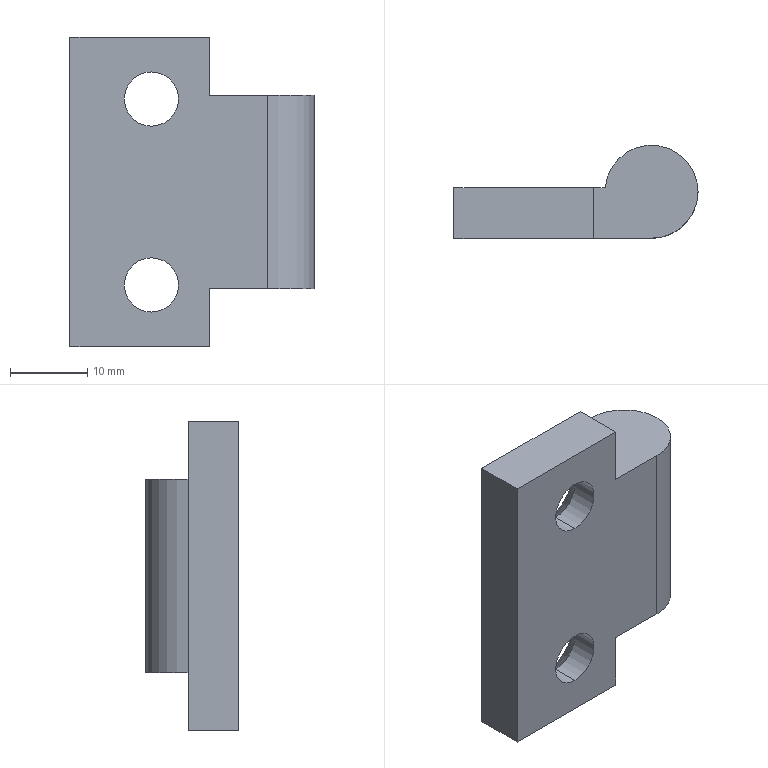Part | SolidWorks | features ICE 3, Chamfer 1, Extrusion 1 | 1 solid | 19 faces | box 31.5 x 12 x 40 mm | volume 7190 mm3 | plane 9 | cylinder 6 | cone 4 | commonest cylinder face diameters 7 x4 12 x2
STEP:
#1=CARTESIAN_POINT('',(-2.24,3.5,-15.5));
#2=VERTEX_POINT('',#1);
#3=CARTESIAN_POINT('',(-2.24,3.5,-8.5));
#4=VERTEX_POINT('',#3);
#5=CARTESIAN_POINT('',(-2.24,3.5,-12.));
#6=DIRECTION('',(0.,1.,0.));
#7=DIRECTION('',(0.,0.,1.));
#8=AXIS2_PLACEMENT_3D('',#5,#6,#7);
#9=CIRCLE('',#8,3.5);
#10=EDGE_CURVE('',#2,#4,#9,.T.);
#11=ORIENTED_EDGE('',*,*,#10,.F.);
#12=CARTESIAN_POINT('',(-2.24,6.5,-18.5));
#13=VERTEX_POINT('',#12);
#14=CARTESIAN_POINT('',(-2.24,3.5,-15.5));
#15=DIRECTION('',(0.,0.7071,-0.7071));
#16=VECTOR('',#15,1000.);
#17=LINE('',#14,#16);
#18=EDGE_CURVE('',#2,#13,#17,.T.);
#19=ORIENTED_EDGE('',*,*,#18,.T.);
#20=CARTESIAN_POINT('',(-2.24,6.5,-5.5));
#21=VERTEX_POINT('',#20);
#22=CARTESIAN_POINT('',(-2.24,6.5,-12.));
#23=DIRECTION('',(0.,-1.,0.));
#24=DIRECTION('',(0.,0.,1.));
#25=AXIS2_PLACEMENT_3D('',#22,#23,#24);
#26=CIRCLE('',#25,6.5);
#27=EDGE_CURVE('',#21,#13,#26,.T.);
#28=ORIENTED_EDGE('',*,*,#27,.F.);
#29=CARTESIAN_POINT('',(-2.24,3.5,-8.5));
#30=DIRECTION('',(0.,0.7071,0.7071));
#31=VECTOR('',#30,1000.);
#32=LINE('',#29,#31);
#33=EDGE_CURVE('',#4,#21,#32,.T.);
#34=ORIENTED_EDGE('',*,*,#33,.F.);
#35=EDGE_LOOP('',(#11,#19,#28,#34));
#36=FACE_OUTER_BOUND('',#35,.T.);
#37=CARTESIAN_POINT('',(-2.24,3.5,-12.));
#38=DIRECTION('',(0.,1.,0.));
#39=DIRECTION('',(0.,0.,1.));
#40=AXIS2_PLACEMENT_3D('',#37,#38,#39);
#41=CONICAL_SURFACE('',#40,3.5,0.7854);
#42=ADVANCED_FACE('',(#36),#41,.F.);
#43=CARTESIAN_POINT('',(-2.24,3.5,8.5));
#44=VERTEX_POINT('',#43);
#45=CARTESIAN_POINT('',(-2.24,3.5,15.5));
#46=VERTEX_POINT('',#45);
#47=CARTESIAN_POINT('',(-2.24,3.5,12.));
#48=DIRECTION('',(0.,1.,0.));
#49=DIRECTION('',(0.,0.,1.));
#50=AXIS2_PLACEMENT_3D('',#47,#48,#49);
#51=CIRCLE('',#50,3.5);
#52=EDGE_CURVE('',#44,#46,#51,.T.);
#53=ORIENTED_EDGE('',*,*,#52,.F.);
#54=CARTESIAN_POINT('',(-2.24,6.5,5.5));
#55=VERTEX_POINT('',#54);
#56=CARTESIAN_POINT('',(-2.24,3.5,8.5));
#57=DIRECTION('',(0.,0.7071,-0.7071));
#58=VECTOR('',#57,1000.);
#59=LINE('',#56,#58);
#60=EDGE_CURVE('',#44,#55,#59,.T.);
#61=ORIENTED_EDGE('',*,*,#60,.T.);
#62=CARTESIAN_POINT('',(-2.24,6.5,18.5));
#63=VERTEX_POINT('',#62);
#64=CARTESIAN_POINT('',(-2.24,6.5,12.));
#65=DIRECTION('',(0.,-1.,0.));
#66=DIRECTION('',(0.,0.,1.));
#67=AXIS2_PLACEMENT_3D('',#64,#65,#66);
#68=CIRCLE('',#67,6.5);
#69=EDGE_CURVE('',#63,#55,#68,.T.);
#70=ORIENTED_EDGE('',*,*,#69,.F.);
#71=CARTESIAN_POINT('',(-2.24,3.5,15.5));
#72=DIRECTION('',(0.,0.7071,0.7071));
#73=VECTOR('',#72,1000.);
#74=LINE('',#71,#73);
#75=EDGE_CURVE('',#46,#63,#74,.T.);
#76=ORIENTED_EDGE('',*,*,#75,.F.);
#77=EDGE_LOOP('',(#53,#61,#70,#76));
#78=FACE_OUTER_BOUND('',#77,.T.);
#79=CARTESIAN_POINT('',(-2.24,3.5,12.));
#80=DIRECTION('',(0.,1.,0.));
#81=DIRECTION('',(0.,0.,1.));
#82=AXIS2_PLACEMENT_3D('',#79,#80,#81);
#83=CONICAL_SURFACE('',#82,3.5,0.7854);
#84=ADVANCED_FACE('',(#78),#83,.F.);
#85=CARTESIAN_POINT('',(-2.24,0.,8.5));
#86=VERTEX_POINT('',#85);
#87=CARTESIAN_POINT('',(-2.24,0.,15.5));
#88=VERTEX_POINT('',#87);
#89=CARTESIAN_POINT('',(-2.24,0.,12.));
#90=DIRECTION('',(0.,1.,0.));
#91=DIRECTION('',(0.,0.,1.));
#92=AXIS2_PLACEMENT_3D('',#89,#90,#91);
#93=CIRCLE('',#92,3.5);
#94=EDGE_CURVE('',#86,#88,#93,.T.);
#95=ORIENTED_EDGE('',*,*,#94,.F.);
#96=CARTESIAN_POINT('',(-2.24,0.,8.5));
#97=DIRECTION('',(0.,1.,0.));
#98=VECTOR('',#97,1000.);
#99=LINE('',#96,#98);
#100=EDGE_CURVE('',#86,#44,#99,.T.);
#101=ORIENTED_EDGE('',*,*,#100,.T.);
#102=ORIENTED_EDGE('',*,*,#52,.T.);
#103=CARTESIAN_POINT('',(-2.24,0.,15.5));
#104=DIRECTION('',(0.,1.,0.));
#105=VECTOR('',#104,1000.);
#106=LINE('',#103,#105);
#107=EDGE_CURVE('',#88,#46,#106,.T.);
#108=ORIENTED_EDGE('',*,*,#107,.F.);
#109=EDGE_LOOP('',(#95,#101,#102,#108));
#110=FACE_OUTER_BOUND('',#109,.T.);
#111=CARTESIAN_POINT('',(-2.24,0.,12.));
#112=DIRECTION('',(0.,1.,0.));
#113=DIRECTION('',(0.,0.,1.));
#114=AXIS2_PLACEMENT_3D('',#111,#112,#113);
#115=CYLINDRICAL_SURFACE('',#114,3.5);
#116=ADVANCED_FACE('',(#110),#115,.F.);
#117=CARTESIAN_POINT('',(-2.24,0.,-15.5));
#118=VERTEX_POINT('',#117);
#119=CARTESIAN_POINT('',(-2.24,0.,-8.5));
#120=VERTEX_POINT('',#119);
#121=CARTESIAN_POINT('',(-2.24,0.,-12.));
#122=DIRECTION('',(0.,1.,0.));
#123=DIRECTION('',(0.,0.,1.));
#124=AXIS2_PLACEMENT_3D('',#121,#122,#123);
#125=CIRCLE('',#124,3.5);
#126=EDGE_CURVE('',#118,#120,#125,.T.);
#127=ORIENTED_EDGE('',*,*,#126,.F.);
#128=CARTESIAN_POINT('',(-2.24,0.,-15.5));
#129=DIRECTION('',(0.,1.,0.));
#130=VECTOR('',#129,1000.);
#131=LINE('',#128,#130);
#132=EDGE_CURVE('',#118,#2,#131,.T.);
#133=ORIENTED_EDGE('',*,*,#132,.T.);
#134=ORIENTED_EDGE('',*,*,#10,.T.);
#135=CARTESIAN_POINT('',(-2.24,0.,-8.5));
#136=DIRECTION('',(0.,1.,0.));
#137=VECTOR('',#136,1000.);
#138=LINE('',#135,#137);
#139=EDGE_CURVE('',#120,#4,#138,.T.);
#140=ORIENTED_EDGE('',*,*,#139,.F.);
#141=EDGE_LOOP('',(#127,#133,#134,#140));
#142=FACE_OUTER_BOUND('',#141,.T.);
#143=CARTESIAN_POINT('',(-2.24,0.,-12.));
#144=DIRECTION('',(0.,1.,0.));
#145=DIRECTION('',(0.,0.,1.));
#146=AXIS2_PLACEMENT_3D('',#143,#144,#145);
#147=CYLINDRICAL_SURFACE('',#146,3.5);
#148=ADVANCED_FACE('',(#142),#147,.F.);
#149=CARTESIAN_POINT('',(18.75,6.,-12.5));
#150=VERTEX_POINT('',#149);
#151=CARTESIAN_POINT('',(12.75,0.,-12.5));
#152=VERTEX_POINT('',#151);
#153=CARTESIAN_POINT('',(12.75,6.,-12.5));
#154=DIRECTION('',(0.,0.,-1.));
#155=DIRECTION('',(1.,0.,0.));
#156=AXIS2_PLACEMENT_3D('',#153,#154,#155);
#157=CIRCLE('',#156,6.);
#158=EDGE_CURVE('',#150,#152,#157,.T.);
#159=ORIENTED_EDGE('',*,*,#158,.F.);
#160=CARTESIAN_POINT('',(18.75,6.,12.5));
#161=VERTEX_POINT('',#160);
#162=CARTESIAN_POINT('',(18.75,6.,-36.971));
#163=DIRECTION('',(0.,0.,1.));
#164=VECTOR('',#163,1000.);
#165=LINE('',#162,#164);
#166=EDGE_CURVE('',#150,#161,#165,.T.);
#167=ORIENTED_EDGE('',*,*,#166,.T.);
#168=CARTESIAN_POINT('',(12.75,0.,12.5));
#169=VERTEX_POINT('',#168);
#170=CARTESIAN_POINT('',(12.75,6.,12.5));
#171=DIRECTION('',(0.,0.,1.));
#172=DIRECTION('',(-1.,0.,0.));
#173=AXIS2_PLACEMENT_3D('',#170,#171,#172);
#174=CIRCLE('',#173,6.);
#175=EDGE_CURVE('',#169,#161,#174,.T.);
#176=ORIENTED_EDGE('',*,*,#175,.F.);
#177=CARTESIAN_POINT('',(12.75,0.,-20.));
#178=DIRECTION('',(0.,0.,-1.));
#179=VECTOR('',#178,1000.);
#180=LINE('',#177,#179);
#181=EDGE_CURVE('',#169,#152,#180,.T.);
#182=ORIENTED_EDGE('',*,*,#181,.T.);
#183=EDGE_LOOP('',(#159,#167,#176,#182));
#184=FACE_OUTER_BOUND('',#183,.T.);
#185=CARTESIAN_POINT('',(12.75,6.,-36.971));
#186=DIRECTION('',(0.,0.,1.));
#187=DIRECTION('',(1.,0.,0.));
#188=AXIS2_PLACEMENT_3D('',#185,#186,#187);
#189=CYLINDRICAL_SURFACE('',#188,6.);
#190=ADVANCED_FACE('',(#184),#189,.T.);
#191=CARTESIAN_POINT('',(5.25,6.5,-20.));
#192=VERTEX_POINT('',#191);
#193=CARTESIAN_POINT('',(-12.75,6.5,-20.));
#194=VERTEX_POINT('',#193);
#195=CARTESIAN_POINT('',(-12.75,6.5,-20.));
#196=DIRECTION('',(-1.,0.,0.));
#197=VECTOR('',#196,1000.);
#198=LINE('',#195,#197);
#199=EDGE_CURVE('',#192,#194,#198,.T.);
#200=ORIENTED_EDGE('',*,*,#199,.F.);
#201=CARTESIAN_POINT('',(5.25,0.,-20.));
#202=VERTEX_POINT('',#201);
#203=CARTESIAN_POINT('',(5.25,12.,-20.));
#204=DIRECTION('',(0.,-1.,0.));
#205=VECTOR('',#204,1000.);
#206=LINE('',#203,#205);
#207=EDGE_CURVE('',#192,#202,#206,.T.);
#208=ORIENTED_EDGE('',*,*,#207,.T.);
#209=CARTESIAN_POINT('',(-12.75,0.,-20.));
#210=VERTEX_POINT('',#209);
#211=CARTESIAN_POINT('',(-12.75,0.,-20.));
#212=DIRECTION('',(-1.,0.,0.));
#213=VECTOR('',#212,1000.);
#214=LINE('',#211,#213);
#215=EDGE_CURVE('',#202,#210,#214,.T.);
#216=ORIENTED_EDGE('',*,*,#215,.T.);
#217=CARTESIAN_POINT('',(-12.75,6.5,-20.));
#218=DIRECTION('',(0.,-1.,0.));
#219=VECTOR('',#218,1000.);
#220=LINE('',#217,#219);
#221=EDGE_CURVE('',#194,#210,#220,.T.);
#222=ORIENTED_EDGE('',*,*,#221,.F.);
#223=EDGE_LOOP('',(#200,#208,#216,#222));
#224=FACE_OUTER_BOUND('',#223,.T.);
#225=CARTESIAN_POINT('',(-12.75,6.5,-20.));
#226=DIRECTION('',(0.,0.,1.));
#227=DIRECTION('',(1.,0.,0.));
#228=AXIS2_PLACEMENT_3D('',#225,#226,#227);
#229=PLANE('',#228);
#230=ADVANCED_FACE('',(#224),#229,.F.);
#231=CARTESIAN_POINT('',(-12.75,0.,20.));
#232=VERTEX_POINT('',#231);
#233=CARTESIAN_POINT('',(-12.75,0.,-20.));
#234=DIRECTION('',(0.,0.,1.));
#235=VECTOR('',#234,1000.);
#236=LINE('',#233,#235);
#237=EDGE_CURVE('',#210,#232,#236,.T.);
#238=ORIENTED_EDGE('',*,*,#237,.T.);
#239=CARTESIAN_POINT('',(-12.75,6.5,20.));
#240=VERTEX_POINT('',#239);
#241=CARTESIAN_POINT('',(-12.75,6.5,20.));
#242=DIRECTION('',(0.,-1.,0.));
#243=VECTOR('',#242,1000.);
#244=LINE('',#241,#243);
#245=EDGE_CURVE('',#240,#232,#244,.T.);
#246=ORIENTED_EDGE('',*,*,#245,.F.);
#247=CARTESIAN_POINT('',(-12.75,6.5,-20.));
#248=DIRECTION('',(0.,0.,1.));
#249=VECTOR('',#248,1000.);
#250=LINE('',#247,#249);
#251=EDGE_CURVE('',#194,#240,#250,.T.);
#252=ORIENTED_EDGE('',*,*,#251,.F.);
#253=ORIENTED_EDGE('',*,*,#221,.T.);
#254=EDGE_LOOP('',(#238,#246,#252,#253));
#255=FACE_OUTER_BOUND('',#254,.T.);
#256=CARTESIAN_POINT('',(-12.75,6.5,-20.));
#257=DIRECTION('',(1.,0.,0.));
#258=DIRECTION('',(0.,0.,-1.));
#259=AXIS2_PLACEMENT_3D('',#256,#257,#258);
#260=PLANE('',#259);
#261=ADVANCED_FACE('',(#255),#260,.F.);
#262=CARTESIAN_POINT('',(5.25,0.,20.));
#263=VERTEX_POINT('',#262);
#264=CARTESIAN_POINT('',(-12.75,0.,20.));
#265=DIRECTION('',(1.,0.,0.));
#266=VECTOR('',#265,1000.);
#267=LINE('',#264,#266);
#268=EDGE_CURVE('',#232,#263,#267,.T.);
#269=ORIENTED_EDGE('',*,*,#268,.T.);
#270=CARTESIAN_POINT('',(5.25,6.5,20.));
#271=VERTEX_POINT('',#270);
#272=CARTESIAN_POINT('',(5.25,12.,20.));
#273=DIRECTION('',(0.,-1.,0.));
#274=VECTOR('',#273,1000.);
#275=LINE('',#272,#274);
#276=EDGE_CURVE('',#271,#263,#275,.T.);
#277=ORIENTED_EDGE('',*,*,#276,.F.);
#278=CARTESIAN_POINT('',(-12.75,6.5,20.));
#279=DIRECTION('',(1.,0.,0.));
#280=VECTOR('',#279,1000.);
#281=LINE('',#278,#280);
#282=EDGE_CURVE('',#240,#271,#281,.T.);
#283=ORIENTED_EDGE('',*,*,#282,.F.);
#284=ORIENTED_EDGE('',*,*,#245,.T.);
#285=EDGE_LOOP('',(#269,#277,#283,#284));
#286=FACE_OUTER_BOUND('',#285,.T.);
#287=CARTESIAN_POINT('',(-12.75,6.5,20.));
#288=DIRECTION('',(0.,0.,-1.));
#289=DIRECTION('',(-1.,0.,0.));
#290=AXIS2_PLACEMENT_3D('',#287,#288,#289);
#291=PLANE('',#290);
#292=ADVANCED_FACE('',(#286),#291,.F.);
#293=ORIENTED_EDGE('',*,*,#69,.T.);
#294=CARTESIAN_POINT('',(-2.24,6.5,12.));
#295=DIRECTION('',(0.,-1.,0.));
#296=DIRECTION('',(0.,0.,1.));
#297=AXIS2_PLACEMENT_3D('',#294,#295,#296);
#298=CIRCLE('',#297,6.5);
#299=EDGE_CURVE('',#55,#63,#298,.T.);
#300=ORIENTED_EDGE('',*,*,#299,.T.);
#301=EDGE_LOOP('',(#293,#300));
#302=FACE_BOUND('',#301,.T.);
#303=ORIENTED_EDGE('',*,*,#27,.T.);
#304=CARTESIAN_POINT('',(-2.24,6.5,-12.));
#305=DIRECTION('',(0.,-1.,0.));
#306=DIRECTION('',(0.,0.,1.));
#307=AXIS2_PLACEMENT_3D('',#304,#305,#306);
#308=CIRCLE('',#307,6.5);
#309=EDGE_CURVE('',#13,#21,#308,.T.);
#310=ORIENTED_EDGE('',*,*,#309,.T.);
#311=EDGE_LOOP('',(#303,#310));
#312=FACE_BOUND('',#311,.T.);
#313=CARTESIAN_POINT('',(5.25,6.5,-12.5));
#314=VERTEX_POINT('',#313);
#315=CARTESIAN_POINT('',(5.25,6.5,0.));
#316=DIRECTION('',(0.,0.,1.));
#317=VECTOR('',#316,1000.);
#318=LINE('',#315,#317);
#319=EDGE_CURVE('',#192,#314,#318,.T.);
#320=ORIENTED_EDGE('',*,*,#319,.F.);
#321=ORIENTED_EDGE('',*,*,#199,.T.);
#322=ORIENTED_EDGE('',*,*,#251,.T.);
#323=ORIENTED_EDGE('',*,*,#282,.T.);
#324=CARTESIAN_POINT('',(5.25,6.5,12.5));
#325=VERTEX_POINT('',#324);
#326=CARTESIAN_POINT('',(5.25,6.5,0.));
#327=DIRECTION('',(0.,0.,1.));
#328=VECTOR('',#327,1000.);
#329=LINE('',#326,#328);
#330=EDGE_CURVE('',#325,#271,#329,.T.);
#331=ORIENTED_EDGE('',*,*,#330,.F.);
#332=CARTESIAN_POINT('',(6.771,6.5,12.5));
#333=VERTEX_POINT('',#332);
#334=CARTESIAN_POINT('',(0.,6.5,12.5));
#335=DIRECTION('',(-1.,0.,0.));
#336=VECTOR('',#335,1000.);
#337=LINE('',#334,#336);
#338=EDGE_CURVE('',#333,#325,#337,.T.);
#339=ORIENTED_EDGE('',*,*,#338,.F.);
#340=CARTESIAN_POINT('',(6.771,6.5,-12.5));
#341=VERTEX_POINT('',#340);
#342=CARTESIAN_POINT('',(6.771,6.5,-36.971));
#343=DIRECTION('',(0.,0.,1.));
#344=VECTOR('',#343,1000.);
#345=LINE('',#342,#344);
#346=EDGE_CURVE('',#341,#333,#345,.T.);
#347=ORIENTED_EDGE('',*,*,#346,.F.);
#348=CARTESIAN_POINT('',(0.,6.5,-12.5));
#349=DIRECTION('',(1.,0.,0.));
#350=VECTOR('',#349,1000.);
#351=LINE('',#348,#350);
#352=EDGE_CURVE('',#314,#341,#351,.T.);
#353=ORIENTED_EDGE('',*,*,#352,.F.);
#354=EDGE_LOOP('',(#320,#321,#322,#323,#331,#339,#347,#353));
#355=FACE_OUTER_BOUND('',#354,.T.);
#356=CARTESIAN_POINT('',(0.,6.5,0.));
#357=DIRECTION('',(0.,1.,0.));
#358=DIRECTION('',(0.,0.,1.));
#359=AXIS2_PLACEMENT_3D('',#356,#357,#358);
#360=PLANE('',#359);
#361=ADVANCED_FACE('',(#302,#312,#355),#360,.T.);
#362=CARTESIAN_POINT('',(-2.24,0.,12.));
#363=DIRECTION('',(0.,1.,0.));
#364=DIRECTION('',(0.,0.,1.));
#365=AXIS2_PLACEMENT_3D('',#362,#363,#364);
#366=CIRCLE('',#365,3.5);
#367=EDGE_CURVE('',#88,#86,#366,.T.);
#368=ORIENTED_EDGE('',*,*,#367,.T.);
#369=ORIENTED_EDGE('',*,*,#94,.T.);
#370=EDGE_LOOP('',(#368,#369));
#371=FACE_BOUND('',#370,.T.);
#372=CARTESIAN_POINT('',(-2.24,0.,-12.));
#373=DIRECTION('',(0.,1.,0.));
#374=DIRECTION('',(0.,0.,1.));
#375=AXIS2_PLACEMENT_3D('',#372,#373,#374);
#376=CIRCLE('',#375,3.5);
#377=EDGE_CURVE('',#120,#118,#376,.T.);
#378=ORIENTED_EDGE('',*,*,#377,.T.);
#379=ORIENTED_EDGE('',*,*,#126,.T.);
#380=EDGE_LOOP('',(#378,#379));
#381=FACE_BOUND('',#380,.T.);
#382=ORIENTED_EDGE('',*,*,#215,.F.);
#383=CARTESIAN_POINT('',(5.25,0.,-12.5));
#384=VERTEX_POINT('',#383);
#385=CARTESIAN_POINT('',(5.25,0.,-20.));
#386=DIRECTION('',(0.,0.,-1.));
#387=VECTOR('',#386,1000.);
#388=LINE('',#385,#387);
#389=EDGE_CURVE('',#384,#202,#388,.T.);
#390=ORIENTED_EDGE('',*,*,#389,.F.);
#391=CARTESIAN_POINT('',(18.75,0.,-12.5));
#392=DIRECTION('',(-1.,0.,0.));
#393=VECTOR('',#392,1000.);
#394=LINE('',#391,#393);
#395=EDGE_CURVE('',#152,#384,#394,.T.);
#396=ORIENTED_EDGE('',*,*,#395,.F.);
#397=ORIENTED_EDGE('',*,*,#181,.F.);
#398=CARTESIAN_POINT('',(5.25,0.,12.5));
#399=VERTEX_POINT('',#398);
#400=CARTESIAN_POINT('',(5.25,0.,12.5));
#401=DIRECTION('',(1.,0.,0.));
#402=VECTOR('',#401,1000.);
#403=LINE('',#400,#402);
#404=EDGE_CURVE('',#399,#169,#403,.T.);
#405=ORIENTED_EDGE('',*,*,#404,.F.);
#406=CARTESIAN_POINT('',(5.25,0.,12.5));
#407=DIRECTION('',(0.,0.,-1.));
#408=VECTOR('',#407,1000.);
#409=LINE('',#406,#408);
#410=EDGE_CURVE('',#263,#399,#409,.T.);
#411=ORIENTED_EDGE('',*,*,#410,.F.);
#412=ORIENTED_EDGE('',*,*,#268,.F.);
#413=ORIENTED_EDGE('',*,*,#237,.F.);
#414=EDGE_LOOP('',(#382,#390,#396,#397,#405,#411,#412,#413));
#415=FACE_OUTER_BOUND('',#414,.T.);
#416=CARTESIAN_POINT('',(0.,0.,0.));
#417=DIRECTION('',(0.,1.,0.));
#418=DIRECTION('',(0.,0.,1.));
#419=AXIS2_PLACEMENT_3D('',#416,#417,#418);
#420=PLANE('',#419);
#421=ADVANCED_FACE('',(#371,#381,#415),#420,.F.);
#422=ORIENTED_EDGE('',*,*,#166,.F.);
#423=CARTESIAN_POINT('',(12.75,6.,-12.5));
#424=DIRECTION('',(0.,0.,-1.));
#425=DIRECTION('',(1.,0.,0.));
#426=AXIS2_PLACEMENT_3D('',#423,#424,#425);
#427=CIRCLE('',#426,6.);
#428=EDGE_CURVE('',#341,#150,#427,.T.);
#429=ORIENTED_EDGE('',*,*,#428,.F.);
#430=ORIENTED_EDGE('',*,*,#346,.T.);
#431=CARTESIAN_POINT('',(12.75,6.,12.5));
#432=DIRECTION('',(0.,0.,1.));
#433=DIRECTION('',(-1.,0.,0.));
#434=AXIS2_PLACEMENT_3D('',#431,#432,#433);
#435=CIRCLE('',#434,6.);
#436=EDGE_CURVE('',#161,#333,#435,.T.);
#437=ORIENTED_EDGE('',*,*,#436,.F.);
#438=EDGE_LOOP('',(#422,#429,#430,#437));
#439=FACE_OUTER_BOUND('',#438,.T.);
#440=CARTESIAN_POINT('',(12.75,6.,-36.971));
#441=DIRECTION('',(0.,0.,1.));
#442=DIRECTION('',(1.,0.,0.));
#443=AXIS2_PLACEMENT_3D('',#440,#441,#442);
#444=CYLINDRICAL_SURFACE('',#443,6.);
#445=ADVANCED_FACE('',(#439),#444,.T.);
#446=ORIENTED_EDGE('',*,*,#330,.T.);
#447=ORIENTED_EDGE('',*,*,#276,.T.);
#448=ORIENTED_EDGE('',*,*,#410,.T.);
#449=CARTESIAN_POINT('',(5.25,12.,12.5));
#450=DIRECTION('',(0.,-1.,0.));
#451=VECTOR('',#450,1000.);
#452=LINE('',#449,#451);
#453=EDGE_CURVE('',#325,#399,#452,.T.);
#454=ORIENTED_EDGE('',*,*,#453,.F.);
#455=EDGE_LOOP('',(#446,#447,#448,#454));
#456=FACE_OUTER_BOUND('',#455,.T.);
#457=CARTESIAN_POINT('',(5.25,12.,12.5));
#458=DIRECTION('',(-1.,0.,0.));
#459=DIRECTION('',(0.,0.,1.));
#460=AXIS2_PLACEMENT_3D('',#457,#458,#459);
#461=PLANE('',#460);
#462=ADVANCED_FACE('',(#456),#461,.F.);
#463=ORIENTED_EDGE('',*,*,#338,.T.);
#464=ORIENTED_EDGE('',*,*,#453,.T.);
#465=ORIENTED_EDGE('',*,*,#404,.T.);
#466=ORIENTED_EDGE('',*,*,#175,.T.);
#467=ORIENTED_EDGE('',*,*,#436,.T.);
#468=EDGE_LOOP('',(#463,#464,#465,#466,#467));
#469=FACE_OUTER_BOUND('',#468,.T.);
#470=CARTESIAN_POINT('',(5.25,12.,12.5));
#471=DIRECTION('',(0.,0.,-1.));
#472=DIRECTION('',(-1.,0.,0.));
#473=AXIS2_PLACEMENT_3D('',#470,#471,#472);
#474=PLANE('',#473);
#475=ADVANCED_FACE('',(#469),#474,.F.);
#476=ORIENTED_EDGE('',*,*,#319,.T.);
#477=CARTESIAN_POINT('',(5.25,12.,-12.5));
#478=DIRECTION('',(0.,-1.,0.));
#479=VECTOR('',#478,1000.);
#480=LINE('',#477,#479);
#481=EDGE_CURVE('',#314,#384,#480,.T.);
#482=ORIENTED_EDGE('',*,*,#481,.T.);
#483=ORIENTED_EDGE('',*,*,#389,.T.);
#484=ORIENTED_EDGE('',*,*,#207,.F.);
#485=EDGE_LOOP('',(#476,#482,#483,#484));
#486=FACE_OUTER_BOUND('',#485,.T.);
#487=CARTESIAN_POINT('',(5.25,12.,-20.));
#488=DIRECTION('',(-1.,0.,0.));
#489=DIRECTION('',(0.,0.,1.));
#490=AXIS2_PLACEMENT_3D('',#487,#488,#489);
#491=PLANE('',#490);
#492=ADVANCED_FACE('',(#486),#491,.F.);
#493=ORIENTED_EDGE('',*,*,#352,.T.);
#494=ORIENTED_EDGE('',*,*,#428,.T.);
#495=ORIENTED_EDGE('',*,*,#158,.T.);
#496=ORIENTED_EDGE('',*,*,#395,.T.);
#497=ORIENTED_EDGE('',*,*,#481,.F.);
#498=EDGE_LOOP('',(#493,#494,#495,#496,#497));
#499=FACE_OUTER_BOUND('',#498,.T.);
#500=CARTESIAN_POINT('',(18.75,12.,-12.5));
#501=DIRECTION('',(0.,0.,1.));
#502=DIRECTION('',(1.,0.,0.));
#503=AXIS2_PLACEMENT_3D('',#500,#501,#502);
#504=PLANE('',#503);
#505=ADVANCED_FACE('',(#499),#504,.F.);
#506=ORIENTED_EDGE('',*,*,#132,.F.);
#507=ORIENTED_EDGE('',*,*,#377,.F.);
#508=ORIENTED_EDGE('',*,*,#139,.T.);
#509=CARTESIAN_POINT('',(-2.24,3.5,-12.));
#510=DIRECTION('',(0.,1.,0.));
#511=DIRECTION('',(0.,0.,1.));
#512=AXIS2_PLACEMENT_3D('',#509,#510,#511);
#513=CIRCLE('',#512,3.5);
#514=EDGE_CURVE('',#4,#2,#513,.T.);
#515=ORIENTED_EDGE('',*,*,#514,.T.);
#516=EDGE_LOOP('',(#506,#507,#508,#515));
#517=FACE_OUTER_BOUND('',#516,.T.);
#518=CARTESIAN_POINT('',(-2.24,0.,-12.));
#519=DIRECTION('',(0.,1.,0.));
#520=DIRECTION('',(0.,0.,1.));
#521=AXIS2_PLACEMENT_3D('',#518,#519,#520);
#522=CYLINDRICAL_SURFACE('',#521,3.5);
#523=ADVANCED_FACE('',(#517),#522,.F.);
#524=ORIENTED_EDGE('',*,*,#100,.F.);
#525=ORIENTED_EDGE('',*,*,#367,.F.);
#526=ORIENTED_EDGE('',*,*,#107,.T.);
#527=CARTESIAN_POINT('',(-2.24,3.5,12.));
#528=DIRECTION('',(0.,1.,0.));
#529=DIRECTION('',(0.,0.,1.));
#530=AXIS2_PLACEMENT_3D('',#527,#528,#529);
#531=CIRCLE('',#530,3.5);
#532=EDGE_CURVE('',#46,#44,#531,.T.);
#533=ORIENTED_EDGE('',*,*,#532,.T.);
#534=EDGE_LOOP('',(#524,#525,#526,#533));
#535=FACE_OUTER_BOUND('',#534,.T.);
#536=CARTESIAN_POINT('',(-2.24,0.,12.));
#537=DIRECTION('',(0.,1.,0.));
#538=DIRECTION('',(0.,0.,1.));
#539=AXIS2_PLACEMENT_3D('',#536,#537,#538);
#540=CYLINDRICAL_SURFACE('',#539,3.5);
#541=ADVANCED_FACE('',(#535),#540,.F.);
#542=ORIENTED_EDGE('',*,*,#60,.F.);
#543=ORIENTED_EDGE('',*,*,#532,.F.);
#544=ORIENTED_EDGE('',*,*,#75,.T.);
#545=ORIENTED_EDGE('',*,*,#299,.F.);
#546=EDGE_LOOP('',(#542,#543,#544,#545));
#547=FACE_OUTER_BOUND('',#546,.T.);
#548=CARTESIAN_POINT('',(-2.24,3.5,12.));
#549=DIRECTION('',(0.,1.,0.));
#550=DIRECTION('',(0.,0.,1.));
#551=AXIS2_PLACEMENT_3D('',#548,#549,#550);
#552=CONICAL_SURFACE('',#551,3.5,0.7854);
#553=ADVANCED_FACE('',(#547),#552,.F.);
#554=ORIENTED_EDGE('',*,*,#18,.F.);
#555=ORIENTED_EDGE('',*,*,#514,.F.);
#556=ORIENTED_EDGE('',*,*,#33,.T.);
#557=ORIENTED_EDGE('',*,*,#309,.F.);
#558=EDGE_LOOP('',(#554,#555,#556,#557));
#559=FACE_OUTER_BOUND('',#558,.T.);
#560=CARTESIAN_POINT('',(-2.24,3.5,-12.));
#561=DIRECTION('',(0.,1.,0.));
#562=DIRECTION('',(0.,0.,1.));
#563=AXIS2_PLACEMENT_3D('',#560,#561,#562);
#564=CONICAL_SURFACE('',#563,3.5,0.7854);
#565=ADVANCED_FACE('',(#559),#564,.F.);
#566=CLOSED_SHELL('',(#42,#84,#116,#148,#190,#230,#261,#292,#361,#421,#445,#462,#475,#492,#505,#523,#541,#553,#565));
#567=MANIFOLD_SOLID_BREP('',#566);
#568=CARTESIAN_POINT('',(0.,0.,0.));
#569=DIRECTION('',(0.,0.,1.));
#570=DIRECTION('',(1.,0.,0.));
#571=AXIS2_PLACEMENT_3D('',#568,#569,#570);
#572=(LENGTH_UNIT()NAMED_UNIT(*)SI_UNIT(.MILLI.,.METRE.));
#573=UNCERTAINTY_MEASURE_WITH_UNIT(LENGTH_MEASURE(0.00001),#572,'','');
#574=(NAMED_UNIT(*)PLANE_ANGLE_UNIT()SI_UNIT($,.RADIAN.));
#575=(NAMED_UNIT(*)SI_UNIT($,.STERADIAN.)SOLID_ANGLE_UNIT());
#576=(GEOMETRIC_REPRESENTATION_CONTEXT(3)GLOBAL_UNCERTAINTY_ASSIGNED_CONTEXT((#573))GLOBAL_UNIT_ASSIGNED_CONTEXT((#572,#574,#575))REPRESENTATION_CONTEXT('',''));
#577=ADVANCED_BREP_SHAPE_REPRESENTATION('',(#567,#571),#576);